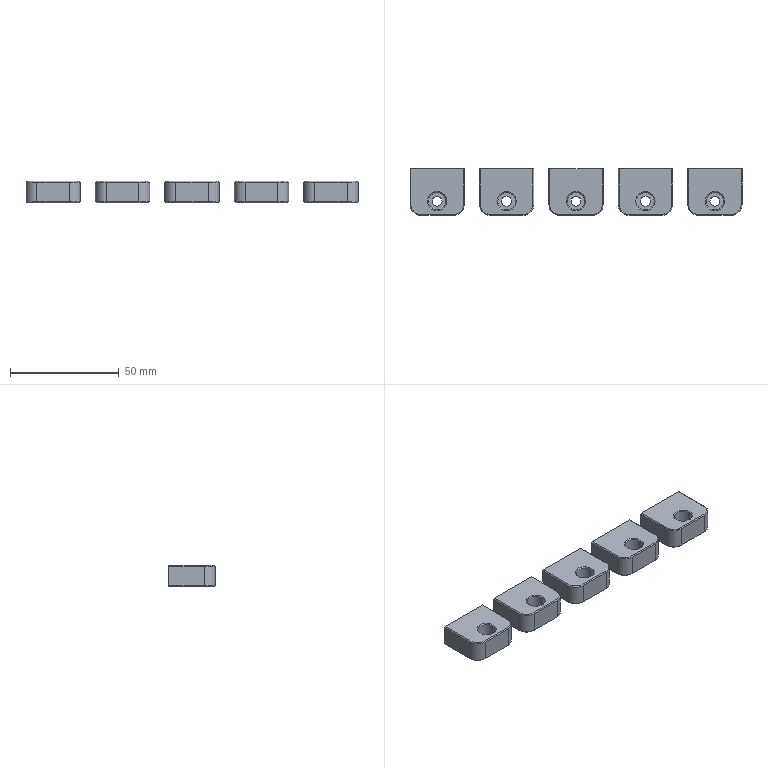NC program | NX | posted with a generic post | part box 153 x 21.5 x 10 mm
Whole program:
N10 G17 G21 G94 G90
(FLOOR_WALL_COPY , TOOL : D63)
N12 T01 M6
N14 G54
N16 G17 G0 G90 X-111. Y0. B0. C0. S6500 M3
N18 G43 Z30. H1
N20 Z7.
N22 G94 G1 Z4. F1250.
N24 X-108.
N26 X108.
N28 X111.
N30 Z7.
N32 G0 Z30.
N34 X-111.
N36 Z6.
N38 G1 Z3.
N40 X-108.
N42 X108.
N44 X111.
N46 Z6.
N48 G0 Z30.
N50 X-111.
N52 Z5.
N54 G1 Z2.
N56 X-108.
N58 X108.
N60 X111.
N62 Z5.
N64 G0 Z30.
N66 X-111.
N68 Z4.
N70 G1 Z1.
N72 X-108.
N74 X108.
N76 X111.
N78 Z4.
N80 G0 Z30.
N82 X-111.
N84 Z3.
N86 G1 Z0.
N88 X-108.
N90 X108.
N92 X111.
N94 Z3.
N96 G0 Z30.
N98 M5
(ZLEVEL_PROFILE_1_COPY_1_COPY_COPY_COPY , TOOL : D4A45)
N100 T02 M6
N102 G54
N104 G17 G0 G90 X63.798 Y-5.118 B0. C0. S9500 M3
N106 G43 Z30. H2
N108 Z0.
N110 G94 G1 Z-1. F1000.
N112 X63.654 Y-5.741
N114 G3 X64. Y-5.941 R0.4
N116 X65.691 Y-4.25 R1.691
N118 X64. Y-5.941 R-1.691
N120 X64.346 Y-5.741 R0.4
N122 G1 X64.202 Y-5.118
N124 Z0.
N126 G0 Z30.
N128 X31.798
N130 Z0.
N132 G1 Z-1.
N134 X31.654 Y-5.741
N136 G3 X32. Y-5.941 R0.4
N138 X33.691 Y-4.25 R1.691
N140 X32. Y-5.941 R-1.691
N142 X32.346 Y-5.741 R0.4
N144 G1 X32.202 Y-5.118
N146 Z0.
N148 G0 Z30.
N150 X-0.202
N152 Z0.
N154 G1 Z-1.
N156 X-0.346 Y-5.741
N158 G3 X0. Y-5.941 R0.4
N160 X1.691 Y-4.25 R1.691
N162 X0. Y-5.941 R-1.691
N164 X0.346 Y-5.741 R0.4
N166 G1 X0.202 Y-5.118
N168 Z0.
N170 G0 Z30.
N172 X-32.202
N174 Z0.
N176 G1 Z-1.
N178 X-32.346 Y-5.741
N180 G3 X-32. Y-5.941 R0.4
N182 X-30.309 Y-4.25 R1.691
N184 X-32. Y-5.941 R-1.691
N186 X-31.654 Y-5.741 R0.4
N188 G1 X-31.798 Y-5.118
N190 Z0.
N192 G0 Z30.
N194 X-64.202
N196 Z0.
N198 G1 Z-1.
N200 X-64.346 Y-5.741
N202 G3 X-64. Y-5.941 R0.4
N204 X-62.309 Y-4.25 R1.691
N206 X-64. Y-5.941 R-1.691
N208 X-63.654 Y-5.741 R0.4
N210 G1 X-63.798 Y-5.118
N212 Z0.
N214 G0 Z30.
N216 X-76.728 Y12.393
N218 Z0.
N220 G1 Z-1.
N222 X-76.448 Y11.909
N224 G3 X-76.102 Y11.709 R0.4
N226 G1 X-51.899
N228 G2 X-50.941 Y10.75 R0.958
N230 G1 Y-5.75
N232 G2 X-56.497 Y-11.309 R5.559
N234 G1 X-71.5
N236 G2 X-77.059 Y-5.75 R5.559
N238 G1 Y10.75
N240 G2 X-76.102 Y11.709 R0.957
N242 G3 X-75.756 Y11.909 R0.4
N244 G1 X-75.41 Y12.509
N246 Z0.
N248 G0 Z30.
N250 X-44.727 Y12.393
N252 Z0.
N254 G1 Z-1.
N256 X-44.447 Y11.909
N258 G3 X-44.101 Y11.709 R0.4
N260 G1 X-19.899
N262 G2 X-18.941 Y10.75 R0.958
N264 G1 Y-5.75
N266 G2 X-24.5 Y-11.309 R5.559
N268 G1 X-39.5
N270 G2 X-45.059 Y-5.75 R5.559
N272 G1 Y10.75
N274 G2 X-44.101 Y11.709 R0.958
N276 G3 X-43.755 Y11.909 R0.4
N278 G1 X-43.409 Y12.509
N280 Z0.
N282 G0 Z30.
N284 X-12.727 Y12.393
N286 Z0.
N288 G1 Z-1.
N290 X-12.447 Y11.909
N292 G3 X-12.101 Y11.709 R0.4
N294 G1 X12.101
N296 G2 X13.059 Y10.75 R0.958
N298 G1 Y-5.75
N300 G2 X7.497 Y-11.309 R5.559
N302 G1 X-7.5
N304 G2 X-13.059 Y-5.75 R5.559
N306 G1 Y10.75
N308 G2 X-12.101 Y11.709 R0.958
N310 G3 X-11.754 Y11.909 R0.4
N312 G1 X-11.408 Y12.509
N314 Z0.
N316 G0 Z30.
N318 X19.273 Y12.393
N320 Z0.
N322 G1 Z-1.
N324 X19.553 Y11.909
N326 G3 X19.899 Y11.709 R0.4
N328 G1 X44.101
N330 G2 X45.059 Y10.75 R0.958
N332 G1 Y-5.75
N334 G2 X39.494 Y-11.309 R5.559
N336 G1 X24.5
N338 G2 X18.941 Y-5.75 R5.559
N340 G1 Y10.75
N342 G2 X19.899 Y11.709 R0.958
N344 G3 X20.246 Y11.909 R0.4
N346 G1 X20.592 Y12.509
N348 Z0.
N350 G0 Z30.
N352 X51.273 Y12.393
N354 Z0.
N356 G1 Z-1.
N358 X51.553 Y11.909
N360 G3 X51.899 Y11.709 R0.4
N362 G1 X76.102
N364 G2 X77.059 Y10.75 R0.957
N366 G1 Y-5.75
N368 G2 X71.504 Y-11.309 R5.559
N370 G1 X56.5
N372 G2 X50.941 Y-5.75 R5.559
N374 G1 Y10.75
N376 G2 X51.899 Y11.709 R0.958
N378 G3 X52.245 Y11.909 R0.4
N380 G1 X52.591 Y12.509
N382 Z0.
N384 G0 Z30.
N386 M5
N388 M2